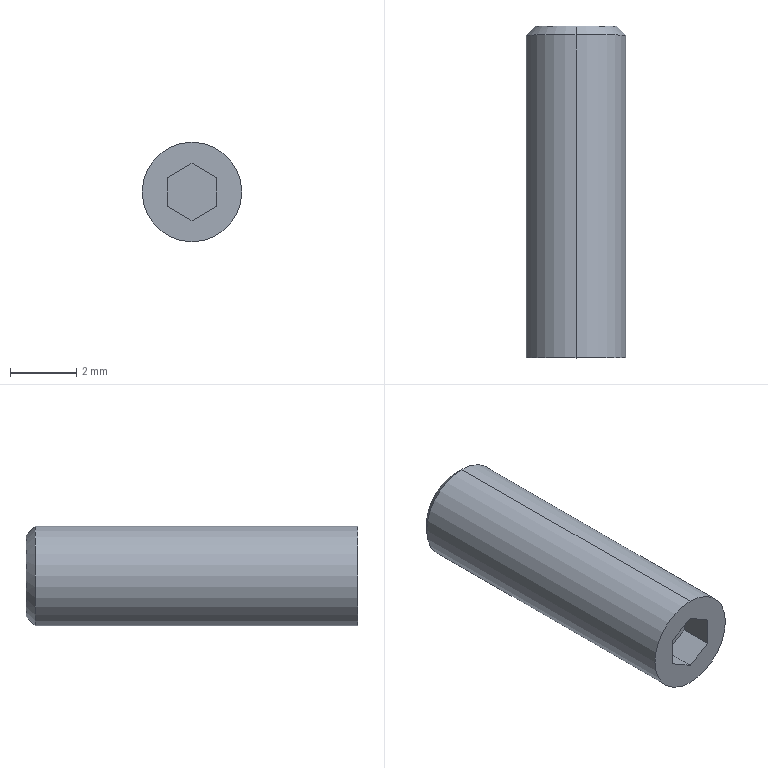Part | SolidWorks | features ICE 2, Extrusion 1, StudWizard 1 | 1 solid | 13 faces | box 3 x 10 x 3 mm | volume 68.413 mm3 | plane 9 | cone 2 | cylinder 2 | commonest cylinder face diameters 3 x2
STEP:
#1=CARTESIAN_POINT('',(0.,10.,-1.23));
#2=VERTEX_POINT('',#1);
#3=CARTESIAN_POINT('',(0.,10.,1.23));
#4=VERTEX_POINT('',#3);
#5=CARTESIAN_POINT('',(0.,10.,0.));
#6=DIRECTION('',(0.,-1.,0.));
#7=DIRECTION('',(0.,0.,-1.));
#8=AXIS2_PLACEMENT_3D('',#5,#6,#7);
#9=CIRCLE('',#8,1.23);
#10=EDGE_CURVE('',#2,#4,#9,.T.);
#11=ORIENTED_EDGE('',*,*,#10,.T.);
#12=CARTESIAN_POINT('',(0.,9.73,1.5));
#13=VERTEX_POINT('',#12);
#14=CARTESIAN_POINT('',(0.,9.73,1.5));
#15=DIRECTION('',(0.,-0.7071,0.7071));
#16=VECTOR('',#15,1000.);
#17=LINE('',#14,#16);
#18=EDGE_CURVE('',#4,#13,#17,.T.);
#19=ORIENTED_EDGE('',*,*,#18,.T.);
#20=CARTESIAN_POINT('',(0.,9.73,-1.5));
#21=VERTEX_POINT('',#20);
#22=CARTESIAN_POINT('',(0.,9.73,0.));
#23=DIRECTION('',(0.,-1.,0.));
#24=DIRECTION('',(0.,0.,-1.));
#25=AXIS2_PLACEMENT_3D('',#22,#23,#24);
#26=CIRCLE('',#25,1.5);
#27=EDGE_CURVE('',#21,#13,#26,.T.);
#28=ORIENTED_EDGE('',*,*,#27,.F.);
#29=CARTESIAN_POINT('',(0.,9.73,-1.5));
#30=DIRECTION('',(0.,-0.7071,-0.7071));
#31=VECTOR('',#30,1000.);
#32=LINE('',#29,#31);
#33=EDGE_CURVE('',#2,#21,#32,.T.);
#34=ORIENTED_EDGE('',*,*,#33,.F.);
#35=EDGE_LOOP('',(#11,#19,#28,#34));
#36=FACE_OUTER_BOUND('',#35,.T.);
#37=CARTESIAN_POINT('',(0.,9.73,0.));
#38=DIRECTION('',(0.,-1.,0.));
#39=DIRECTION('',(0.,0.,-1.));
#40=AXIS2_PLACEMENT_3D('',#37,#38,#39);
#41=CONICAL_SURFACE('',#40,1.5,0.7854);
#42=ADVANCED_FACE('',(#36),#41,.T.);
#43=CARTESIAN_POINT('',(0.,0.,-1.5));
#44=VERTEX_POINT('',#43);
#45=CARTESIAN_POINT('',(0.,0.,1.5));
#46=VERTEX_POINT('',#45);
#47=CARTESIAN_POINT('',(0.,0.,0.));
#48=DIRECTION('',(0.,-1.,0.));
#49=DIRECTION('',(0.,0.,-1.));
#50=AXIS2_PLACEMENT_3D('',#47,#48,#49);
#51=CIRCLE('',#50,1.5);
#52=EDGE_CURVE('',#44,#46,#51,.T.);
#53=ORIENTED_EDGE('',*,*,#52,.F.);
#54=CARTESIAN_POINT('',(0.,-1.,-1.5));
#55=DIRECTION('',(0.,1.,0.));
#56=VECTOR('',#55,1000.);
#57=LINE('',#54,#56);
#58=EDGE_CURVE('',#44,#21,#57,.T.);
#59=ORIENTED_EDGE('',*,*,#58,.T.);
#60=ORIENTED_EDGE('',*,*,#27,.T.);
#61=CARTESIAN_POINT('',(0.,-1.,1.5));
#62=DIRECTION('',(0.,1.,0.));
#63=VECTOR('',#62,1000.);
#64=LINE('',#61,#63);
#65=EDGE_CURVE('',#46,#13,#64,.T.);
#66=ORIENTED_EDGE('',*,*,#65,.F.);
#67=EDGE_LOOP('',(#53,#59,#60,#66));
#68=FACE_OUTER_BOUND('',#67,.T.);
#69=CARTESIAN_POINT('',(0.,-1.,0.));
#70=DIRECTION('',(0.,1.,0.));
#71=DIRECTION('',(0.,0.,1.));
#72=AXIS2_PLACEMENT_3D('',#69,#70,#71);
#73=CYLINDRICAL_SURFACE('',#72,1.5);
#74=ADVANCED_FACE('',(#68),#73,.T.);
#75=ORIENTED_EDGE('',*,*,#58,.F.);
#76=CARTESIAN_POINT('',(0.,0.,0.));
#77=DIRECTION('',(0.,-1.,0.));
#78=DIRECTION('',(0.,0.,-1.));
#79=AXIS2_PLACEMENT_3D('',#76,#77,#78);
#80=CIRCLE('',#79,1.5);
#81=EDGE_CURVE('',#46,#44,#80,.T.);
#82=ORIENTED_EDGE('',*,*,#81,.F.);
#83=ORIENTED_EDGE('',*,*,#65,.T.);
#84=CARTESIAN_POINT('',(0.,9.73,0.));
#85=DIRECTION('',(0.,-1.,0.));
#86=DIRECTION('',(0.,0.,-1.));
#87=AXIS2_PLACEMENT_3D('',#84,#85,#86);
#88=CIRCLE('',#87,1.5);
#89=EDGE_CURVE('',#13,#21,#88,.T.);
#90=ORIENTED_EDGE('',*,*,#89,.T.);
#91=EDGE_LOOP('',(#75,#82,#83,#90));
#92=FACE_OUTER_BOUND('',#91,.T.);
#93=CARTESIAN_POINT('',(0.,-1.,0.));
#94=DIRECTION('',(0.,1.,0.));
#95=DIRECTION('',(0.,0.,1.));
#96=AXIS2_PLACEMENT_3D('',#93,#94,#95);
#97=CYLINDRICAL_SURFACE('',#96,1.5);
#98=ADVANCED_FACE('',(#92),#97,.T.);
#99=ORIENTED_EDGE('',*,*,#10,.F.);
#100=CARTESIAN_POINT('',(0.,10.,0.));
#101=DIRECTION('',(0.,-1.,0.));
#102=DIRECTION('',(0.,0.,-1.));
#103=AXIS2_PLACEMENT_3D('',#100,#101,#102);
#104=CIRCLE('',#103,1.23);
#105=EDGE_CURVE('',#4,#2,#104,.T.);
#106=ORIENTED_EDGE('',*,*,#105,.F.);
#107=EDGE_LOOP('',(#99,#106));
#108=FACE_OUTER_BOUND('',#107,.T.);
#109=CARTESIAN_POINT('',(1.23,10.,0.));
#110=DIRECTION('',(0.,1.,0.));
#111=DIRECTION('',(0.,0.,1.));
#112=AXIS2_PLACEMENT_3D('',#109,#110,#111);
#113=PLANE('',#112);
#114=ADVANCED_FACE('',(#108),#113,.T.);
#115=ORIENTED_EDGE('',*,*,#18,.F.);
#116=ORIENTED_EDGE('',*,*,#105,.T.);
#117=ORIENTED_EDGE('',*,*,#33,.T.);
#118=ORIENTED_EDGE('',*,*,#89,.F.);
#119=EDGE_LOOP('',(#115,#116,#117,#118));
#120=FACE_OUTER_BOUND('',#119,.T.);
#121=CARTESIAN_POINT('',(0.,9.73,0.));
#122=DIRECTION('',(0.,-1.,0.));
#123=DIRECTION('',(0.,0.,-1.));
#124=AXIS2_PLACEMENT_3D('',#121,#122,#123);
#125=CONICAL_SURFACE('',#124,1.5,0.7854);
#126=ADVANCED_FACE('',(#120),#125,.T.);
#127=CARTESIAN_POINT('',(0.75,0.,0.433));
#128=VERTEX_POINT('',#127);
#129=CARTESIAN_POINT('',(0.,0.,0.866));
#130=VERTEX_POINT('',#129);
#131=CARTESIAN_POINT('',(0.75,0.,0.433));
#132=DIRECTION('',(-0.866,0.,0.5));
#133=VECTOR('',#132,1000.);
#134=LINE('',#131,#133);
#135=EDGE_CURVE('',#128,#130,#134,.T.);
#136=ORIENTED_EDGE('',*,*,#135,.F.);
#137=CARTESIAN_POINT('',(0.75,0.,-0.433));
#138=VERTEX_POINT('',#137);
#139=CARTESIAN_POINT('',(0.75,0.,-0.433));
#140=DIRECTION('',(0.,0.,1.));
#141=VECTOR('',#140,1000.);
#142=LINE('',#139,#141);
#143=EDGE_CURVE('',#138,#128,#142,.T.);
#144=ORIENTED_EDGE('',*,*,#143,.F.);
#145=CARTESIAN_POINT('',(0.,0.,-0.866));
#146=VERTEX_POINT('',#145);
#147=CARTESIAN_POINT('',(0.,0.,-0.866));
#148=DIRECTION('',(0.866,0.,0.5));
#149=VECTOR('',#148,1000.);
#150=LINE('',#147,#149);
#151=EDGE_CURVE('',#146,#138,#150,.T.);
#152=ORIENTED_EDGE('',*,*,#151,.F.);
#153=CARTESIAN_POINT('',(-0.75,0.,-0.433));
#154=VERTEX_POINT('',#153);
#155=CARTESIAN_POINT('',(-0.75,0.,-0.433));
#156=DIRECTION('',(0.866,0.,-0.5));
#157=VECTOR('',#156,1000.);
#158=LINE('',#155,#157);
#159=EDGE_CURVE('',#154,#146,#158,.T.);
#160=ORIENTED_EDGE('',*,*,#159,.F.);
#161=CARTESIAN_POINT('',(-0.75,0.,0.433));
#162=VERTEX_POINT('',#161);
#163=CARTESIAN_POINT('',(-0.75,0.,0.433));
#164=DIRECTION('',(0.,0.,-1.));
#165=VECTOR('',#164,1000.);
#166=LINE('',#163,#165);
#167=EDGE_CURVE('',#162,#154,#166,.T.);
#168=ORIENTED_EDGE('',*,*,#167,.F.);
#169=CARTESIAN_POINT('',(0.,0.,0.866));
#170=DIRECTION('',(-0.866,0.,-0.5));
#171=VECTOR('',#170,1000.);
#172=LINE('',#169,#171);
#173=EDGE_CURVE('',#130,#162,#172,.T.);
#174=ORIENTED_EDGE('',*,*,#173,.F.);
#175=EDGE_LOOP('',(#136,#144,#152,#160,#168,#174));
#176=FACE_BOUND('',#175,.T.);
#177=ORIENTED_EDGE('',*,*,#81,.T.);
#178=ORIENTED_EDGE('',*,*,#52,.T.);
#179=EDGE_LOOP('',(#177,#178));
#180=FACE_OUTER_BOUND('',#179,.T.);
#181=CARTESIAN_POINT('',(0.,0.,0.));
#182=DIRECTION('',(0.,-1.,0.));
#183=DIRECTION('',(0.,0.,-1.));
#184=AXIS2_PLACEMENT_3D('',#181,#182,#183);
#185=PLANE('',#184);
#186=ADVANCED_FACE('',(#176,#180),#185,.T.);
#187=ORIENTED_EDGE('',*,*,#135,.T.);
#188=CARTESIAN_POINT('',(0.,1.,0.866));
#189=VERTEX_POINT('',#188);
#190=CARTESIAN_POINT('',(0.,1.,0.866));
#191=DIRECTION('',(0.,-1.,0.));
#192=VECTOR('',#191,1000.);
#193=LINE('',#190,#192);
#194=EDGE_CURVE('',#189,#130,#193,.T.);
#195=ORIENTED_EDGE('',*,*,#194,.F.);
#196=CARTESIAN_POINT('',(0.75,1.,0.433));
#197=VERTEX_POINT('',#196);
#198=CARTESIAN_POINT('',(0.75,1.,0.433));
#199=DIRECTION('',(-0.866,0.,0.5));
#200=VECTOR('',#199,1000.);
#201=LINE('',#198,#200);
#202=EDGE_CURVE('',#197,#189,#201,.T.);
#203=ORIENTED_EDGE('',*,*,#202,.F.);
#204=CARTESIAN_POINT('',(0.75,1.,0.433));
#205=DIRECTION('',(0.,-1.,0.));
#206=VECTOR('',#205,1000.);
#207=LINE('',#204,#206);
#208=EDGE_CURVE('',#197,#128,#207,.T.);
#209=ORIENTED_EDGE('',*,*,#208,.T.);
#210=EDGE_LOOP('',(#187,#195,#203,#209));
#211=FACE_OUTER_BOUND('',#210,.T.);
#212=CARTESIAN_POINT('',(0.75,1.,0.433));
#213=DIRECTION('',(0.5,0.,0.866));
#214=DIRECTION('',(0.866,0.,-0.5));
#215=AXIS2_PLACEMENT_3D('',#212,#213,#214);
#216=PLANE('',#215);
#217=ADVANCED_FACE('',(#211),#216,.F.);
#218=ORIENTED_EDGE('',*,*,#143,.T.);
#219=ORIENTED_EDGE('',*,*,#208,.F.);
#220=CARTESIAN_POINT('',(0.75,1.,-0.433));
#221=VERTEX_POINT('',#220);
#222=CARTESIAN_POINT('',(0.75,1.,-0.433));
#223=DIRECTION('',(0.,0.,1.));
#224=VECTOR('',#223,1000.);
#225=LINE('',#222,#224);
#226=EDGE_CURVE('',#221,#197,#225,.T.);
#227=ORIENTED_EDGE('',*,*,#226,.F.);
#228=CARTESIAN_POINT('',(0.75,1.,-0.433));
#229=DIRECTION('',(0.,-1.,0.));
#230=VECTOR('',#229,1000.);
#231=LINE('',#228,#230);
#232=EDGE_CURVE('',#221,#138,#231,.T.);
#233=ORIENTED_EDGE('',*,*,#232,.T.);
#234=EDGE_LOOP('',(#218,#219,#227,#233));
#235=FACE_OUTER_BOUND('',#234,.T.);
#236=CARTESIAN_POINT('',(0.75,1.,-0.433));
#237=DIRECTION('',(1.,0.,0.));
#238=DIRECTION('',(0.,0.,-1.));
#239=AXIS2_PLACEMENT_3D('',#236,#237,#238);
#240=PLANE('',#239);
#241=ADVANCED_FACE('',(#235),#240,.F.);
#242=ORIENTED_EDGE('',*,*,#151,.T.);
#243=ORIENTED_EDGE('',*,*,#232,.F.);
#244=CARTESIAN_POINT('',(0.,1.,-0.866));
#245=VERTEX_POINT('',#244);
#246=CARTESIAN_POINT('',(0.,1.,-0.866));
#247=DIRECTION('',(0.866,0.,0.5));
#248=VECTOR('',#247,1000.);
#249=LINE('',#246,#248);
#250=EDGE_CURVE('',#245,#221,#249,.T.);
#251=ORIENTED_EDGE('',*,*,#250,.F.);
#252=CARTESIAN_POINT('',(0.,1.,-0.866));
#253=DIRECTION('',(0.,-1.,0.));
#254=VECTOR('',#253,1000.);
#255=LINE('',#252,#254);
#256=EDGE_CURVE('',#245,#146,#255,.T.);
#257=ORIENTED_EDGE('',*,*,#256,.T.);
#258=EDGE_LOOP('',(#242,#243,#251,#257));
#259=FACE_OUTER_BOUND('',#258,.T.);
#260=CARTESIAN_POINT('',(0.,1.,-0.866));
#261=DIRECTION('',(0.5,0.,-0.866));
#262=DIRECTION('',(-0.866,0.,-0.5));
#263=AXIS2_PLACEMENT_3D('',#260,#261,#262);
#264=PLANE('',#263);
#265=ADVANCED_FACE('',(#259),#264,.F.);
#266=ORIENTED_EDGE('',*,*,#159,.T.);
#267=ORIENTED_EDGE('',*,*,#256,.F.);
#268=CARTESIAN_POINT('',(-0.75,1.,-0.433));
#269=VERTEX_POINT('',#268);
#270=CARTESIAN_POINT('',(-0.75,1.,-0.433));
#271=DIRECTION('',(0.866,0.,-0.5));
#272=VECTOR('',#271,1000.);
#273=LINE('',#270,#272);
#274=EDGE_CURVE('',#269,#245,#273,.T.);
#275=ORIENTED_EDGE('',*,*,#274,.F.);
#276=CARTESIAN_POINT('',(-0.75,1.,-0.433));
#277=DIRECTION('',(0.,-1.,0.));
#278=VECTOR('',#277,1000.);
#279=LINE('',#276,#278);
#280=EDGE_CURVE('',#269,#154,#279,.T.);
#281=ORIENTED_EDGE('',*,*,#280,.T.);
#282=EDGE_LOOP('',(#266,#267,#275,#281));
#283=FACE_OUTER_BOUND('',#282,.T.);
#284=CARTESIAN_POINT('',(-0.75,1.,-0.433));
#285=DIRECTION('',(-0.5,0.,-0.866));
#286=DIRECTION('',(-0.866,0.,0.5));
#287=AXIS2_PLACEMENT_3D('',#284,#285,#286);
#288=PLANE('',#287);
#289=ADVANCED_FACE('',(#283),#288,.F.);
#290=ORIENTED_EDGE('',*,*,#167,.T.);
#291=ORIENTED_EDGE('',*,*,#280,.F.);
#292=CARTESIAN_POINT('',(-0.75,1.,0.433));
#293=VERTEX_POINT('',#292);
#294=CARTESIAN_POINT('',(-0.75,1.,0.433));
#295=DIRECTION('',(0.,0.,-1.));
#296=VECTOR('',#295,1000.);
#297=LINE('',#294,#296);
#298=EDGE_CURVE('',#293,#269,#297,.T.);
#299=ORIENTED_EDGE('',*,*,#298,.F.);
#300=CARTESIAN_POINT('',(-0.75,1.,0.433));
#301=DIRECTION('',(0.,-1.,0.));
#302=VECTOR('',#301,1000.);
#303=LINE('',#300,#302);
#304=EDGE_CURVE('',#293,#162,#303,.T.);
#305=ORIENTED_EDGE('',*,*,#304,.T.);
#306=EDGE_LOOP('',(#290,#291,#299,#305));
#307=FACE_OUTER_BOUND('',#306,.T.);
#308=CARTESIAN_POINT('',(-0.75,1.,0.433));
#309=DIRECTION('',(-1.,0.,0.));
#310=DIRECTION('',(0.,0.,1.));
#311=AXIS2_PLACEMENT_3D('',#308,#309,#310);
#312=PLANE('',#311);
#313=ADVANCED_FACE('',(#307),#312,.F.);
#314=ORIENTED_EDGE('',*,*,#173,.T.);
#315=ORIENTED_EDGE('',*,*,#304,.F.);
#316=CARTESIAN_POINT('',(0.,1.,0.866));
#317=DIRECTION('',(-0.866,0.,-0.5));
#318=VECTOR('',#317,1000.);
#319=LINE('',#316,#318);
#320=EDGE_CURVE('',#189,#293,#319,.T.);
#321=ORIENTED_EDGE('',*,*,#320,.F.);
#322=ORIENTED_EDGE('',*,*,#194,.T.);
#323=EDGE_LOOP('',(#314,#315,#321,#322));
#324=FACE_OUTER_BOUND('',#323,.T.);
#325=CARTESIAN_POINT('',(0.,1.,0.866));
#326=DIRECTION('',(-0.5,0.,0.866));
#327=DIRECTION('',(0.866,0.,0.5));
#328=AXIS2_PLACEMENT_3D('',#325,#326,#327);
#329=PLANE('',#328);
#330=ADVANCED_FACE('',(#324),#329,.F.);
#331=ORIENTED_EDGE('',*,*,#202,.T.);
#332=ORIENTED_EDGE('',*,*,#320,.T.);
#333=ORIENTED_EDGE('',*,*,#298,.T.);
#334=ORIENTED_EDGE('',*,*,#274,.T.);
#335=ORIENTED_EDGE('',*,*,#250,.T.);
#336=ORIENTED_EDGE('',*,*,#226,.T.);
#337=EDGE_LOOP('',(#331,#332,#333,#334,#335,#336));
#338=FACE_OUTER_BOUND('',#337,.T.);
#339=CARTESIAN_POINT('',(0.,1.,0.));
#340=DIRECTION('',(0.,-1.,0.));
#341=DIRECTION('',(0.,0.,-1.));
#342=AXIS2_PLACEMENT_3D('',#339,#340,#341);
#343=PLANE('',#342);
#344=ADVANCED_FACE('',(#338),#343,.T.);
#345=CLOSED_SHELL('',(#42,#74,#98,#114,#126,#186,#217,#241,#265,#289,#313,#330,#344));
#346=MANIFOLD_SOLID_BREP('',#345);
#347=CARTESIAN_POINT('',(0.,0.,0.));
#348=DIRECTION('',(0.,0.,1.));
#349=DIRECTION('',(1.,0.,0.));
#350=AXIS2_PLACEMENT_3D('',#347,#348,#349);
#351=(LENGTH_UNIT()NAMED_UNIT(*)SI_UNIT(.MILLI.,.METRE.));
#352=UNCERTAINTY_MEASURE_WITH_UNIT(LENGTH_MEASURE(0.00001),#351,'','');
#353=(NAMED_UNIT(*)PLANE_ANGLE_UNIT()SI_UNIT($,.RADIAN.));
#354=(NAMED_UNIT(*)SI_UNIT($,.STERADIAN.)SOLID_ANGLE_UNIT());
#355=(GEOMETRIC_REPRESENTATION_CONTEXT(3)GLOBAL_UNCERTAINTY_ASSIGNED_CONTEXT((#352))GLOBAL_UNIT_ASSIGNED_CONTEXT((#351,#353,#354))REPRESENTATION_CONTEXT('',''));
#356=ADVANCED_BREP_SHAPE_REPRESENTATION('',(#346,#350),#355);